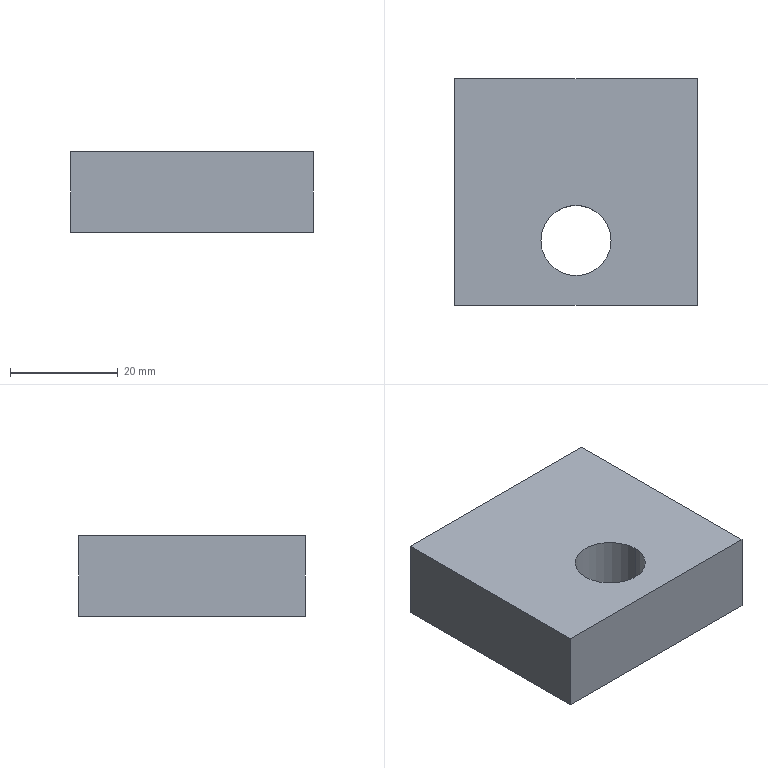Part | STEP file | adjusting block_default | 1 solid | 16 faces | box 45 x 42 x 15 mm | volume 24875 mm3 | cylinder 6 | plane 6 | cone 4 | commonest cylinder face diameters 6.8 x4 13 x2
STEP:
#1=CARTESIAN_POINT('',(0.,0.,0.));
#2=DIRECTION('',(0.,0.,1.));
#3=DIRECTION('',(1.,0.,0.));
#4=AXIS2_PLACEMENT_3D('',#1,#2,#3);
#5=CARTESIAN_POINT('',(29.,-30.,0.));
#6=VERTEX_POINT('',#5);
#7=CARTESIAN_POINT('',(29.,-30.,15.));
#8=VERTEX_POINT('',#7);
#9=CARTESIAN_POINT('',(29.,-30.,15.));
#10=DIRECTION('',(0.,0.,1.));
#11=VECTOR('',#10,1.);
#12=LINE('',#9,#11);
#13=CARTESIAN_POINT('',(22.5,-30.,15.));
#14=DIRECTION('',(0.,0.,1.));
#15=DIRECTION('',(1.,0.,0.));
#16=AXIS2_PLACEMENT_3D('',#13,#14,#15);
#17=CYLINDRICAL_SURFACE('',#16,6.5);
#18=CARTESIAN_POINT('',(6.283,0.));
#19=DIRECTION('',(0.,1.));
#20=VECTOR('',#19,1.);
#21=LINE('',#18,#20);
#22=(GEOMETRIC_REPRESENTATION_CONTEXT(2)PARAMETRIC_REPRESENTATION_CONTEXT()REPRESENTATION_CONTEXT('',''));
#23=DEFINITIONAL_REPRESENTATION('',(#21),#22);
#24=PCURVE('',#17,#23);
#25=CARTESIAN_POINT('',(22.5,-30.,15.));
#26=DIRECTION('',(0.,0.,1.));
#27=DIRECTION('',(1.,0.,0.));
#28=AXIS2_PLACEMENT_3D('',#25,#26,#27);
#29=CYLINDRICAL_SURFACE('',#28,6.5);
#30=CARTESIAN_POINT('',(0.,0.));
#31=DIRECTION('',(0.,1.));
#32=VECTOR('',#31,1.);
#33=LINE('',#30,#32);
#34=(GEOMETRIC_REPRESENTATION_CONTEXT(2)PARAMETRIC_REPRESENTATION_CONTEXT()REPRESENTATION_CONTEXT('',''));
#35=DEFINITIONAL_REPRESENTATION('',(#33),#34);
#36=PCURVE('',#29,#35);
#37=SURFACE_CURVE('',#12,(#24,#36),.PCURVE_S1.);
#38=EDGE_CURVE('',#6,#8,#37,.T.);
#39=ORIENTED_EDGE('',*,*,#38,.T.);
#40=CARTESIAN_POINT('',(16.,-30.,15.));
#41=VERTEX_POINT('',#40);
#42=CARTESIAN_POINT('',(22.5,-30.,15.));
#43=DIRECTION('',(0.,0.,1.));
#44=DIRECTION('',(1.,0.,0.));
#45=AXIS2_PLACEMENT_3D('',#42,#43,#44);
#46=CIRCLE('',#45,6.5);
#47=CARTESIAN_POINT('',(0.,0.));
#48=DIRECTION('',(1.,0.));
#49=VECTOR('',#48,1.);
#50=LINE('',#47,#49);
#51=(GEOMETRIC_REPRESENTATION_CONTEXT(2)PARAMETRIC_REPRESENTATION_CONTEXT()REPRESENTATION_CONTEXT('',''));
#52=DEFINITIONAL_REPRESENTATION('',(#50),#51);
#53=PCURVE('',#17,#52);
#54=CARTESIAN_POINT('',(0.,0.,15.));
#55=DIRECTION('',(0.,0.,1.));
#56=DIRECTION('',(1.,0.,0.));
#57=AXIS2_PLACEMENT_3D('',#54,#55,#56);
#58=PLANE('',#57);
#59=CARTESIAN_POINT('',(22.5,-30.));
#60=DIRECTION('',(1.,0.));
#61=AXIS2_PLACEMENT_2D('',#59,#60);
#62=CIRCLE('',#61,6.5);
#63=(GEOMETRIC_REPRESENTATION_CONTEXT(2)PARAMETRIC_REPRESENTATION_CONTEXT()REPRESENTATION_CONTEXT('',''));
#64=DEFINITIONAL_REPRESENTATION('',(#62),#63);
#65=PCURVE('',#58,#64);
#66=SURFACE_CURVE('',#46,(#53,#65),.PCURVE_S1.);
#67=EDGE_CURVE('',#41,#8,#66,.T.);
#68=ORIENTED_EDGE('',*,*,#67,.F.);
#69=CARTESIAN_POINT('',(16.,-30.,0.));
#70=VERTEX_POINT('',#69);
#71=CARTESIAN_POINT('',(16.,-30.,15.));
#72=DIRECTION('',(0.,0.,1.));
#73=VECTOR('',#72,1.);
#74=LINE('',#71,#73);
#75=CARTESIAN_POINT('',(3.142,0.));
#76=DIRECTION('',(0.,1.));
#77=VECTOR('',#76,1.);
#78=LINE('',#75,#77);
#79=(GEOMETRIC_REPRESENTATION_CONTEXT(2)PARAMETRIC_REPRESENTATION_CONTEXT()REPRESENTATION_CONTEXT('',''));
#80=DEFINITIONAL_REPRESENTATION('',(#78),#79);
#81=PCURVE('',#17,#80);
#82=CARTESIAN_POINT('',(3.142,0.));
#83=DIRECTION('',(0.,1.));
#84=VECTOR('',#83,1.);
#85=LINE('',#82,#84);
#86=(GEOMETRIC_REPRESENTATION_CONTEXT(2)PARAMETRIC_REPRESENTATION_CONTEXT()REPRESENTATION_CONTEXT('',''));
#87=DEFINITIONAL_REPRESENTATION('',(#85),#86);
#88=PCURVE('',#29,#87);
#89=SURFACE_CURVE('',#74,(#81,#88),.PCURVE_S1.);
#90=EDGE_CURVE('',#70,#41,#89,.T.);
#91=ORIENTED_EDGE('',*,*,#90,.F.);
#92=CARTESIAN_POINT('',(22.5,-30.,0.));
#93=DIRECTION('',(0.,0.,1.));
#94=DIRECTION('',(1.,0.,0.));
#95=AXIS2_PLACEMENT_3D('',#92,#93,#94);
#96=CIRCLE('',#95,6.5);
#97=CARTESIAN_POINT('',(0.,-15.));
#98=DIRECTION('',(1.,0.));
#99=VECTOR('',#98,1.);
#100=LINE('',#97,#99);
#101=(GEOMETRIC_REPRESENTATION_CONTEXT(2)PARAMETRIC_REPRESENTATION_CONTEXT()REPRESENTATION_CONTEXT('',''));
#102=DEFINITIONAL_REPRESENTATION('',(#100),#101);
#103=PCURVE('',#17,#102);
#104=CARTESIAN_POINT('',(0.,0.,0.));
#105=DIRECTION('',(0.,0.,1.));
#106=DIRECTION('',(1.,0.,0.));
#107=AXIS2_PLACEMENT_3D('',#104,#105,#106);
#108=PLANE('',#107);
#109=CARTESIAN_POINT('',(22.5,-30.));
#110=DIRECTION('',(1.,0.));
#111=AXIS2_PLACEMENT_2D('',#109,#110);
#112=CIRCLE('',#111,6.5);
#113=(GEOMETRIC_REPRESENTATION_CONTEXT(2)PARAMETRIC_REPRESENTATION_CONTEXT()REPRESENTATION_CONTEXT('',''));
#114=DEFINITIONAL_REPRESENTATION('',(#112),#113);
#115=PCURVE('',#108,#114);
#116=SURFACE_CURVE('',#96,(#103,#115),.PCURVE_S1.);
#117=EDGE_CURVE('',#70,#6,#116,.T.);
#118=ORIENTED_EDGE('',*,*,#117,.T.);
#119=EDGE_LOOP('',(#39,#68,#91,#118));
#120=FACE_BOUND('',#119,.F.);
#121=ADVANCED_FACE('',(#120),#17,.F.);
#122=CARTESIAN_POINT('',(7.5,-19.75,10.9));
#123=VERTEX_POINT('',#122);
#124=CARTESIAN_POINT('',(7.5,0.,10.9));
#125=VERTEX_POINT('',#124);
#126=CARTESIAN_POINT('',(7.5,0.,10.9));
#127=DIRECTION('',(0.,1.,0.));
#128=VECTOR('',#127,1.);
#129=LINE('',#126,#128);
#130=CARTESIAN_POINT('',(7.5,0.,7.5));
#131=DIRECTION('',(0.,1.,0.));
#132=DIRECTION('',(0.,0.,1.));
#133=AXIS2_PLACEMENT_3D('',#130,#131,#132);
#134=CYLINDRICAL_SURFACE('',#133,3.4);
#135=CARTESIAN_POINT('',(6.283,0.));
#136=DIRECTION('',(0.,1.));
#137=VECTOR('',#136,1.);
#138=LINE('',#135,#137);
#139=(GEOMETRIC_REPRESENTATION_CONTEXT(2)PARAMETRIC_REPRESENTATION_CONTEXT()REPRESENTATION_CONTEXT('',''));
#140=DEFINITIONAL_REPRESENTATION('',(#138),#139);
#141=PCURVE('',#134,#140);
#142=CARTESIAN_POINT('',(7.5,0.,7.5));
#143=DIRECTION('',(0.,1.,0.));
#144=DIRECTION('',(0.,0.,1.));
#145=AXIS2_PLACEMENT_3D('',#142,#143,#144);
#146=CYLINDRICAL_SURFACE('',#145,3.4);
#147=CARTESIAN_POINT('',(0.,0.));
#148=DIRECTION('',(0.,1.));
#149=VECTOR('',#148,1.);
#150=LINE('',#147,#149);
#151=(GEOMETRIC_REPRESENTATION_CONTEXT(2)PARAMETRIC_REPRESENTATION_CONTEXT()REPRESENTATION_CONTEXT('',''));
#152=DEFINITIONAL_REPRESENTATION('',(#150),#151);
#153=PCURVE('',#146,#152);
#154=SURFACE_CURVE('',#129,(#141,#153),.PCURVE_S1.);
#155=EDGE_CURVE('',#123,#125,#154,.T.);
#156=ORIENTED_EDGE('',*,*,#155,.T.);
#157=CARTESIAN_POINT('',(7.5,0.,4.1));
#158=VERTEX_POINT('',#157);
#159=CARTESIAN_POINT('',(7.5,0.,7.5));
#160=DIRECTION('',(0.,1.,0.));
#161=DIRECTION('',(0.,0.,1.));
#162=AXIS2_PLACEMENT_3D('',#159,#160,#161);
#163=CIRCLE('',#162,3.4);
#164=CARTESIAN_POINT('',(0.,0.));
#165=DIRECTION('',(1.,0.));
#166=VECTOR('',#165,1.);
#167=LINE('',#164,#166);
#168=(GEOMETRIC_REPRESENTATION_CONTEXT(2)PARAMETRIC_REPRESENTATION_CONTEXT()REPRESENTATION_CONTEXT('',''));
#169=DEFINITIONAL_REPRESENTATION('',(#167),#168);
#170=PCURVE('',#134,#169);
#171=CARTESIAN_POINT('',(0.,0.,15.));
#172=DIRECTION('',(0.,-1.,0.));
#173=DIRECTION('',(0.,0.,-1.));
#174=AXIS2_PLACEMENT_3D('',#171,#172,#173);
#175=PLANE('',#174);
#176=CARTESIAN_POINT('',(4.1,7.5));
#177=CARTESIAN_POINT('',(4.1,13.389));
#178=CARTESIAN_POINT('',(9.2,10.444));
#179=CARTESIAN_POINT('',(14.3,7.5));
#180=CARTESIAN_POINT('',(9.2,4.556));
#181=CARTESIAN_POINT('',(4.1,1.611));
#182=CARTESIAN_POINT('',(4.1,7.5));
#183=(BOUNDED_CURVE()B_SPLINE_CURVE(2,(#176,#177,#178,#179,#180,#181,#182),.UNSPECIFIED.,.T.,.F.)B_SPLINE_CURVE_WITH_KNOTS((1,2,2,2,2,1),(-2.094,0.,2.094,4.189,6.283,8.378),.UNSPECIFIED.)CURVE()GEOMETRIC_REPRESENTATION_ITEM()RATIONAL_B_SPLINE_CURVE((1.,0.5,1.,0.5,1.,0.5,1.))REPRESENTATION_ITEM(''));
#184=(GEOMETRIC_REPRESENTATION_CONTEXT(2)PARAMETRIC_REPRESENTATION_CONTEXT()REPRESENTATION_CONTEXT('',''));
#185=DEFINITIONAL_REPRESENTATION('',(#183),#184);
#186=PCURVE('',#175,#185);
#187=SURFACE_CURVE('',#163,(#170,#186),.PCURVE_S1.);
#188=EDGE_CURVE('',#158,#125,#187,.T.);
#189=ORIENTED_EDGE('',*,*,#188,.F.);
#190=CARTESIAN_POINT('',(7.5,-19.75,4.1));
#191=VERTEX_POINT('',#190);
#192=CARTESIAN_POINT('',(7.5,0.,4.1));
#193=DIRECTION('',(0.,1.,0.));
#194=VECTOR('',#193,1.);
#195=LINE('',#192,#194);
#196=CARTESIAN_POINT('',(3.142,0.));
#197=DIRECTION('',(0.,1.));
#198=VECTOR('',#197,1.);
#199=LINE('',#196,#198);
#200=(GEOMETRIC_REPRESENTATION_CONTEXT(2)PARAMETRIC_REPRESENTATION_CONTEXT()REPRESENTATION_CONTEXT('',''));
#201=DEFINITIONAL_REPRESENTATION('',(#199),#200);
#202=PCURVE('',#134,#201);
#203=CARTESIAN_POINT('',(3.142,0.));
#204=DIRECTION('',(0.,1.));
#205=VECTOR('',#204,1.);
#206=LINE('',#203,#205);
#207=(GEOMETRIC_REPRESENTATION_CONTEXT(2)PARAMETRIC_REPRESENTATION_CONTEXT()REPRESENTATION_CONTEXT('',''));
#208=DEFINITIONAL_REPRESENTATION('',(#206),#207);
#209=PCURVE('',#146,#208);
#210=SURFACE_CURVE('',#195,(#202,#209),.PCURVE_S1.);
#211=EDGE_CURVE('',#191,#158,#210,.T.);
#212=ORIENTED_EDGE('',*,*,#211,.F.);
#213=CARTESIAN_POINT('',(7.5,-19.75,7.5));
#214=DIRECTION('',(0.,1.,0.));
#215=DIRECTION('',(0.,0.,1.));
#216=AXIS2_PLACEMENT_3D('',#213,#214,#215);
#217=CIRCLE('',#216,3.4);
#218=CARTESIAN_POINT('',(0.,-19.75));
#219=DIRECTION('',(1.,0.));
#220=VECTOR('',#219,1.);
#221=LINE('',#218,#220);
#222=(GEOMETRIC_REPRESENTATION_CONTEXT(2)PARAMETRIC_REPRESENTATION_CONTEXT()REPRESENTATION_CONTEXT('',''));
#223=DEFINITIONAL_REPRESENTATION('',(#221),#222);
#224=PCURVE('',#134,#223);
#225=CARTESIAN_POINT('',(7.5,-19.75,7.5));
#226=DIRECTION('',(0.,1.,0.));
#227=DIRECTION('',(0.,0.,1.));
#228=AXIS2_PLACEMENT_3D('',#225,#226,#227);
#229=CONICAL_SURFACE('',#228,3.4,1.03);
#230=CARTESIAN_POINT('',(0.,0.));
#231=DIRECTION('',(1.,0.));
#232=VECTOR('',#231,1.);
#233=LINE('',#230,#232);
#234=(GEOMETRIC_REPRESENTATION_CONTEXT(2)PARAMETRIC_REPRESENTATION_CONTEXT()REPRESENTATION_CONTEXT('',''));
#235=DEFINITIONAL_REPRESENTATION('',(#233),#234);
#236=PCURVE('',#229,#235);
#237=SURFACE_CURVE('',#217,(#224,#236),.PCURVE_S1.);
#238=EDGE_CURVE('',#191,#123,#237,.T.);
#239=ORIENTED_EDGE('',*,*,#238,.T.);
#240=EDGE_LOOP('',(#156,#189,#212,#239));
#241=FACE_BOUND('',#240,.F.);
#242=ADVANCED_FACE('',(#241),#134,.F.);
#243=ORIENTED_EDGE('',*,*,#238,.F.);
#244=CARTESIAN_POINT('',(7.5,-21.793,7.5));
#245=VERTEX_POINT('',#244);
#246=CARTESIAN_POINT('',(7.5,-19.75,4.1));
#247=DIRECTION('',(0.,0.515,-0.8572));
#248=VECTOR('',#247,1.);
#249=LINE('',#246,#248);
#250=CARTESIAN_POINT('',(3.142,0.));
#251=DIRECTION('',(0.,1.));
#252=VECTOR('',#251,1.);
#253=LINE('',#250,#252);
#254=(GEOMETRIC_REPRESENTATION_CONTEXT(2)PARAMETRIC_REPRESENTATION_CONTEXT()REPRESENTATION_CONTEXT('',''));
#255=DEFINITIONAL_REPRESENTATION('',(#253),#254);
#256=PCURVE('',#229,#255);
#257=CARTESIAN_POINT('',(7.5,-19.75,7.5));
#258=DIRECTION('',(0.,1.,0.));
#259=DIRECTION('',(0.,0.,1.));
#260=AXIS2_PLACEMENT_3D('',#257,#258,#259);
#261=CONICAL_SURFACE('',#260,3.4,1.03);
#262=CARTESIAN_POINT('',(3.142,0.));
#263=DIRECTION('',(0.,1.));
#264=VECTOR('',#263,1.);
#265=LINE('',#262,#264);
#266=(GEOMETRIC_REPRESENTATION_CONTEXT(2)PARAMETRIC_REPRESENTATION_CONTEXT()REPRESENTATION_CONTEXT('',''));
#267=DEFINITIONAL_REPRESENTATION('',(#265),#266);
#268=PCURVE('',#261,#267);
#269=SURFACE_CURVE('',#249,(#256,#268),.PCURVE_S1.);
#270=EDGE_CURVE('',#245,#191,#269,.T.);
#271=ORIENTED_EDGE('',*,*,#270,.F.);
#272=CARTESIAN_POINT('',(7.5,-19.75,10.9));
#273=DIRECTION('',(0.,0.515,0.8572));
#274=VECTOR('',#273,1.);
#275=LINE('',#272,#274);
#276=CARTESIAN_POINT('',(6.283,0.));
#277=DIRECTION('',(0.,1.));
#278=VECTOR('',#277,1.);
#279=LINE('',#276,#278);
#280=(GEOMETRIC_REPRESENTATION_CONTEXT(2)PARAMETRIC_REPRESENTATION_CONTEXT()REPRESENTATION_CONTEXT('',''));
#281=DEFINITIONAL_REPRESENTATION('',(#279),#280);
#282=PCURVE('',#229,#281);
#283=CARTESIAN_POINT('',(0.,0.));
#284=DIRECTION('',(0.,1.));
#285=VECTOR('',#284,1.);
#286=LINE('',#283,#285);
#287=(GEOMETRIC_REPRESENTATION_CONTEXT(2)PARAMETRIC_REPRESENTATION_CONTEXT()REPRESENTATION_CONTEXT('',''));
#288=DEFINITIONAL_REPRESENTATION('',(#286),#287);
#289=PCURVE('',#261,#288);
#290=SURFACE_CURVE('',#275,(#282,#289),.PCURVE_S1.);
#291=EDGE_CURVE('',#245,#123,#290,.T.);
#292=ORIENTED_EDGE('',*,*,#291,.T.);
#293=EDGE_LOOP('',(#243,#271,#292));
#294=FACE_BOUND('',#293,.F.);
#295=ADVANCED_FACE('',(#294),#229,.F.);
#296=CARTESIAN_POINT('',(37.5,-19.75,10.9));
#297=VERTEX_POINT('',#296);
#298=CARTESIAN_POINT('',(37.5,0.,10.9));
#299=VERTEX_POINT('',#298);
#300=CARTESIAN_POINT('',(37.5,0.,10.9));
#301=DIRECTION('',(0.,1.,0.));
#302=VECTOR('',#301,1.);
#303=LINE('',#300,#302);
#304=CARTESIAN_POINT('',(37.5,0.,7.5));
#305=DIRECTION('',(0.,1.,0.));
#306=DIRECTION('',(0.,0.,1.));
#307=AXIS2_PLACEMENT_3D('',#304,#305,#306);
#308=CYLINDRICAL_SURFACE('',#307,3.4);
#309=CARTESIAN_POINT('',(6.283,0.));
#310=DIRECTION('',(0.,1.));
#311=VECTOR('',#310,1.);
#312=LINE('',#309,#311);
#313=(GEOMETRIC_REPRESENTATION_CONTEXT(2)PARAMETRIC_REPRESENTATION_CONTEXT()REPRESENTATION_CONTEXT('',''));
#314=DEFINITIONAL_REPRESENTATION('',(#312),#313);
#315=PCURVE('',#308,#314);
#316=CARTESIAN_POINT('',(37.5,0.,7.5));
#317=DIRECTION('',(0.,1.,0.));
#318=DIRECTION('',(0.,0.,1.));
#319=AXIS2_PLACEMENT_3D('',#316,#317,#318);
#320=CYLINDRICAL_SURFACE('',#319,3.4);
#321=CARTESIAN_POINT('',(0.,0.));
#322=DIRECTION('',(0.,1.));
#323=VECTOR('',#322,1.);
#324=LINE('',#321,#323);
#325=(GEOMETRIC_REPRESENTATION_CONTEXT(2)PARAMETRIC_REPRESENTATION_CONTEXT()REPRESENTATION_CONTEXT('',''));
#326=DEFINITIONAL_REPRESENTATION('',(#324),#325);
#327=PCURVE('',#320,#326);
#328=SURFACE_CURVE('',#303,(#315,#327),.PCURVE_S1.);
#329=EDGE_CURVE('',#297,#299,#328,.T.);
#330=ORIENTED_EDGE('',*,*,#329,.T.);
#331=CARTESIAN_POINT('',(37.5,0.,4.1));
#332=VERTEX_POINT('',#331);
#333=CARTESIAN_POINT('',(37.5,0.,7.5));
#334=DIRECTION('',(0.,1.,0.));
#335=DIRECTION('',(0.,0.,1.));
#336=AXIS2_PLACEMENT_3D('',#333,#334,#335);
#337=CIRCLE('',#336,3.4);
#338=CARTESIAN_POINT('',(0.,0.));
#339=DIRECTION('',(1.,0.));
#340=VECTOR('',#339,1.);
#341=LINE('',#338,#340);
#342=(GEOMETRIC_REPRESENTATION_CONTEXT(2)PARAMETRIC_REPRESENTATION_CONTEXT()REPRESENTATION_CONTEXT('',''));
#343=DEFINITIONAL_REPRESENTATION('',(#341),#342);
#344=PCURVE('',#308,#343);
#345=CARTESIAN_POINT('',(4.1,37.5));
#346=CARTESIAN_POINT('',(4.1,43.389));
#347=CARTESIAN_POINT('',(9.2,40.444));
#348=CARTESIAN_POINT('',(14.3,37.5));
#349=CARTESIAN_POINT('',(9.2,34.556));
#350=CARTESIAN_POINT('',(4.1,31.611));
#351=CARTESIAN_POINT('',(4.1,37.5));
#352=(BOUNDED_CURVE()B_SPLINE_CURVE(2,(#345,#346,#347,#348,#349,#350,#351),.UNSPECIFIED.,.T.,.F.)B_SPLINE_CURVE_WITH_KNOTS((1,2,2,2,2,1),(-2.094,0.,2.094,4.189,6.283,8.378),.UNSPECIFIED.)CURVE()GEOMETRIC_REPRESENTATION_ITEM()RATIONAL_B_SPLINE_CURVE((1.,0.5,1.,0.5,1.,0.5,1.))REPRESENTATION_ITEM(''));
#353=(GEOMETRIC_REPRESENTATION_CONTEXT(2)PARAMETRIC_REPRESENTATION_CONTEXT()REPRESENTATION_CONTEXT('',''));
#354=DEFINITIONAL_REPRESENTATION('',(#352),#353);
#355=PCURVE('',#175,#354);
#356=SURFACE_CURVE('',#337,(#344,#355),.PCURVE_S1.);
#357=EDGE_CURVE('',#332,#299,#356,.T.);
#358=ORIENTED_EDGE('',*,*,#357,.F.);
#359=CARTESIAN_POINT('',(37.5,-19.75,4.1));
#360=VERTEX_POINT('',#359);
#361=CARTESIAN_POINT('',(37.5,0.,4.1));
#362=DIRECTION('',(0.,1.,0.));
#363=VECTOR('',#362,1.);
#364=LINE('',#361,#363);
#365=CARTESIAN_POINT('',(3.142,0.));
#366=DIRECTION('',(0.,1.));
#367=VECTOR('',#366,1.);
#368=LINE('',#365,#367);
#369=(GEOMETRIC_REPRESENTATION_CONTEXT(2)PARAMETRIC_REPRESENTATION_CONTEXT()REPRESENTATION_CONTEXT('',''));
#370=DEFINITIONAL_REPRESENTATION('',(#368),#369);
#371=PCURVE('',#308,#370);
#372=CARTESIAN_POINT('',(3.142,0.));
#373=DIRECTION('',(0.,1.));
#374=VECTOR('',#373,1.);
#375=LINE('',#372,#374);
#376=(GEOMETRIC_REPRESENTATION_CONTEXT(2)PARAMETRIC_REPRESENTATION_CONTEXT()REPRESENTATION_CONTEXT('',''));
#377=DEFINITIONAL_REPRESENTATION('',(#375),#376);
#378=PCURVE('',#320,#377);
#379=SURFACE_CURVE('',#364,(#371,#378),.PCURVE_S1.);
#380=EDGE_CURVE('',#360,#332,#379,.T.);
#381=ORIENTED_EDGE('',*,*,#380,.F.);
#382=CARTESIAN_POINT('',(37.5,-19.75,7.5));
#383=DIRECTION('',(0.,1.,0.));
#384=DIRECTION('',(0.,0.,1.));
#385=AXIS2_PLACEMENT_3D('',#382,#383,#384);
#386=CIRCLE('',#385,3.4);
#387=CARTESIAN_POINT('',(0.,-19.75));
#388=DIRECTION('',(1.,0.));
#389=VECTOR('',#388,1.);
#390=LINE('',#387,#389);
#391=(GEOMETRIC_REPRESENTATION_CONTEXT(2)PARAMETRIC_REPRESENTATION_CONTEXT()REPRESENTATION_CONTEXT('',''));
#392=DEFINITIONAL_REPRESENTATION('',(#390),#391);
#393=PCURVE('',#308,#392);
#394=CARTESIAN_POINT('',(37.5,-19.75,7.5));
#395=DIRECTION('',(0.,1.,0.));
#396=DIRECTION('',(0.,0.,1.));
#397=AXIS2_PLACEMENT_3D('',#394,#395,#396);
#398=CONICAL_SURFACE('',#397,3.4,1.03);
#399=CARTESIAN_POINT('',(0.,0.));
#400=DIRECTION('',(1.,0.));
#401=VECTOR('',#400,1.);
#402=LINE('',#399,#401);
#403=(GEOMETRIC_REPRESENTATION_CONTEXT(2)PARAMETRIC_REPRESENTATION_CONTEXT()REPRESENTATION_CONTEXT('',''));
#404=DEFINITIONAL_REPRESENTATION('',(#402),#403);
#405=PCURVE('',#398,#404);
#406=SURFACE_CURVE('',#386,(#393,#405),.PCURVE_S1.);
#407=EDGE_CURVE('',#360,#297,#406,.T.);
#408=ORIENTED_EDGE('',*,*,#407,.T.);
#409=EDGE_LOOP('',(#330,#358,#381,#408));
#410=FACE_BOUND('',#409,.F.);
#411=ADVANCED_FACE('',(#410),#308,.F.);
#412=ORIENTED_EDGE('',*,*,#407,.F.);
#413=CARTESIAN_POINT('',(37.5,-21.793,7.5));
#414=VERTEX_POINT('',#413);
#415=CARTESIAN_POINT('',(37.5,-19.75,4.1));
#416=DIRECTION('',(0.,0.515,-0.8572));
#417=VECTOR('',#416,1.);
#418=LINE('',#415,#417);
#419=CARTESIAN_POINT('',(3.142,0.));
#420=DIRECTION('',(0.,1.));
#421=VECTOR('',#420,1.);
#422=LINE('',#419,#421);
#423=(GEOMETRIC_REPRESENTATION_CONTEXT(2)PARAMETRIC_REPRESENTATION_CONTEXT()REPRESENTATION_CONTEXT('',''));
#424=DEFINITIONAL_REPRESENTATION('',(#422),#423);
#425=PCURVE('',#398,#424);
#426=CARTESIAN_POINT('',(37.5,-19.75,7.5));
#427=DIRECTION('',(0.,1.,0.));
#428=DIRECTION('',(0.,0.,1.));
#429=AXIS2_PLACEMENT_3D('',#426,#427,#428);
#430=CONICAL_SURFACE('',#429,3.4,1.03);
#431=CARTESIAN_POINT('',(3.142,0.));
#432=DIRECTION('',(0.,1.));
#433=VECTOR('',#432,1.);
#434=LINE('',#431,#433);
#435=(GEOMETRIC_REPRESENTATION_CONTEXT(2)PARAMETRIC_REPRESENTATION_CONTEXT()REPRESENTATION_CONTEXT('',''));
#436=DEFINITIONAL_REPRESENTATION('',(#434),#435);
#437=PCURVE('',#430,#436);
#438=SURFACE_CURVE('',#418,(#425,#437),.PCURVE_S1.);
#439=EDGE_CURVE('',#414,#360,#438,.T.);
#440=ORIENTED_EDGE('',*,*,#439,.F.);
#441=CARTESIAN_POINT('',(37.5,-19.75,10.9));
#442=DIRECTION('',(0.,0.515,0.8572));
#443=VECTOR('',#442,1.);
#444=LINE('',#441,#443);
#445=CARTESIAN_POINT('',(6.283,0.));
#446=DIRECTION('',(0.,1.));
#447=VECTOR('',#446,1.);
#448=LINE('',#445,#447);
#449=(GEOMETRIC_REPRESENTATION_CONTEXT(2)PARAMETRIC_REPRESENTATION_CONTEXT()REPRESENTATION_CONTEXT('',''));
#450=DEFINITIONAL_REPRESENTATION('',(#448),#449);
#451=PCURVE('',#398,#450);
#452=CARTESIAN_POINT('',(0.,0.));
#453=DIRECTION('',(0.,1.));
#454=VECTOR('',#453,1.);
#455=LINE('',#452,#454);
#456=(GEOMETRIC_REPRESENTATION_CONTEXT(2)PARAMETRIC_REPRESENTATION_CONTEXT()REPRESENTATION_CONTEXT('',''));
#457=DEFINITIONAL_REPRESENTATION('',(#455),#456);
#458=PCURVE('',#430,#457);
#459=SURFACE_CURVE('',#444,(#451,#458),.PCURVE_S1.);
#460=EDGE_CURVE('',#414,#297,#459,.T.);
#461=ORIENTED_EDGE('',*,*,#460,.T.);
#462=EDGE_LOOP('',(#412,#440,#461));
#463=FACE_BOUND('',#462,.F.);
#464=ADVANCED_FACE('',(#463),#398,.F.);
#465=CARTESIAN_POINT('',(0.,0.,0.));
#466=VERTEX_POINT('',#465);
#467=CARTESIAN_POINT('',(0.,-42.,0.));
#468=VERTEX_POINT('',#467);
#469=CARTESIAN_POINT('',(0.,0.,0.));
#470=DIRECTION('',(0.,-1.,0.));
#471=VECTOR('',#470,1.);
#472=LINE('',#469,#471);
#473=CARTESIAN_POINT('',(0.,0.,15.));
#474=DIRECTION('',(1.,0.,0.));
#475=DIRECTION('',(0.,1.,0.));
#476=AXIS2_PLACEMENT_3D('',#473,#474,#475);
#477=PLANE('',#476);
#478=CARTESIAN_POINT('',(0.,-15.));
#479=DIRECTION('',(-1.,0.));
#480=VECTOR('',#479,1.);
#481=LINE('',#478,#480);
#482=(GEOMETRIC_REPRESENTATION_CONTEXT(2)PARAMETRIC_REPRESENTATION_CONTEXT()REPRESENTATION_CONTEXT('',''));
#483=DEFINITIONAL_REPRESENTATION('',(#481),#482);
#484=PCURVE('',#477,#483);
#485=CARTESIAN_POINT('',(0.,0.));
#486=DIRECTION('',(0.,-1.));
#487=VECTOR('',#486,1.);
#488=LINE('',#485,#487);
#489=(GEOMETRIC_REPRESENTATION_CONTEXT(2)PARAMETRIC_REPRESENTATION_CONTEXT()REPRESENTATION_CONTEXT('',''));
#490=DEFINITIONAL_REPRESENTATION('',(#488),#489);
#491=PCURVE('',#108,#490);
#492=SURFACE_CURVE('',#472,(#484,#491),.PCURVE_S1.);
#493=EDGE_CURVE('',#466,#468,#492,.T.);
#494=ORIENTED_EDGE('',*,*,#493,.T.);
#495=CARTESIAN_POINT('',(0.,-42.,15.));
#496=VERTEX_POINT('',#495);
#497=CARTESIAN_POINT('',(0.,-42.,15.));
#498=DIRECTION('',(0.,0.,-1.));
#499=VECTOR('',#498,1.);
#500=LINE('',#497,#499);
#501=CARTESIAN_POINT('',(-42.,0.));
#502=DIRECTION('',(0.,-1.));
#503=VECTOR('',#502,1.);
#504=LINE('',#501,#503);
#505=(GEOMETRIC_REPRESENTATION_CONTEXT(2)PARAMETRIC_REPRESENTATION_CONTEXT()REPRESENTATION_CONTEXT('',''));
#506=DEFINITIONAL_REPRESENTATION('',(#504),#505);
#507=PCURVE('',#477,#506);
#508=CARTESIAN_POINT('',(0.,-42.,15.));
#509=DIRECTION('',(0.,1.,0.));
#510=DIRECTION('',(0.,0.,1.));
#511=AXIS2_PLACEMENT_3D('',#508,#509,#510);
#512=PLANE('',#511);
#513=CARTESIAN_POINT('',(0.,0.));
#514=DIRECTION('',(-1.,0.));
#515=VECTOR('',#514,1.);
#516=LINE('',#513,#515);
#517=(GEOMETRIC_REPRESENTATION_CONTEXT(2)PARAMETRIC_REPRESENTATION_CONTEXT()REPRESENTATION_CONTEXT('',''));
#518=DEFINITIONAL_REPRESENTATION('',(#516),#517);
#519=PCURVE('',#512,#518);
#520=SURFACE_CURVE('',#500,(#507,#519),.PCURVE_S1.);
#521=EDGE_CURVE('',#496,#468,#520,.T.);
#522=ORIENTED_EDGE('',*,*,#521,.F.);
#523=CARTESIAN_POINT('',(0.,0.,15.));
#524=VERTEX_POINT('',#523);
#525=CARTESIAN_POINT('',(0.,0.,15.));
#526=DIRECTION('',(0.,-1.,0.));
#527=VECTOR('',#526,1.);
#528=LINE('',#525,#527);
#529=CARTESIAN_POINT('',(0.,0.));
#530=DIRECTION('',(-1.,0.));
#531=VECTOR('',#530,1.);
#532=LINE('',#529,#531);
#533=(GEOMETRIC_REPRESENTATION_CONTEXT(2)PARAMETRIC_REPRESENTATION_CONTEXT()REPRESENTATION_CONTEXT('',''));
#534=DEFINITIONAL_REPRESENTATION('',(#532),#533);
#535=PCURVE('',#477,#534);
#536=CARTESIAN_POINT('',(0.,0.));
#537=DIRECTION('',(0.,-1.));
#538=VECTOR('',#537,1.);
#539=LINE('',#536,#538);
#540=(GEOMETRIC_REPRESENTATION_CONTEXT(2)PARAMETRIC_REPRESENTATION_CONTEXT()REPRESENTATION_CONTEXT('',''));
#541=DEFINITIONAL_REPRESENTATION('',(#539),#540);
#542=PCURVE('',#58,#541);
#543=SURFACE_CURVE('',#528,(#535,#542),.PCURVE_S1.);
#544=EDGE_CURVE('',#524,#496,#543,.T.);
#545=ORIENTED_EDGE('',*,*,#544,.F.);
#546=CARTESIAN_POINT('',(0.,0.,15.));
#547=DIRECTION('',(0.,0.,-1.));
#548=VECTOR('',#547,1.);
#549=LINE('',#546,#548);
#550=CARTESIAN_POINT('',(0.,0.));
#551=DIRECTION('',(0.,-1.));
#552=VECTOR('',#551,1.);
#553=LINE('',#550,#552);
#554=(GEOMETRIC_REPRESENTATION_CONTEXT(2)PARAMETRIC_REPRESENTATION_CONTEXT()REPRESENTATION_CONTEXT('',''));
#555=DEFINITIONAL_REPRESENTATION('',(#553),#554);
#556=PCURVE('',#477,#555);
#557=CARTESIAN_POINT('',(0.,0.));
#558=DIRECTION('',(1.,0.));
#559=VECTOR('',#558,1.);
#560=LINE('',#557,#559);
#561=(GEOMETRIC_REPRESENTATION_CONTEXT(2)PARAMETRIC_REPRESENTATION_CONTEXT()REPRESENTATION_CONTEXT('',''));
#562=DEFINITIONAL_REPRESENTATION('',(#560),#561);
#563=PCURVE('',#175,#562);
#564=SURFACE_CURVE('',#549,(#556,#563),.PCURVE_S1.);
#565=EDGE_CURVE('',#524,#466,#564,.T.);
#566=ORIENTED_EDGE('',*,*,#565,.T.);
#567=EDGE_LOOP('',(#494,#522,#545,#566));
#568=FACE_BOUND('',#567,.T.);
#569=ADVANCED_FACE('',(#568),#477,.F.);
#570=CARTESIAN_POINT('',(45.,-42.,0.));
#571=VERTEX_POINT('',#570);
#572=CARTESIAN_POINT('',(0.,-42.,0.));
#573=DIRECTION('',(1.,0.,0.));
#574=VECTOR('',#573,1.);
#575=LINE('',#572,#574);
#576=CARTESIAN_POINT('',(-15.,0.));
#577=DIRECTION('',(0.,1.));
#578=VECTOR('',#577,1.);
#579=LINE('',#576,#578);
#580=(GEOMETRIC_REPRESENTATION_CONTEXT(2)PARAMETRIC_REPRESENTATION_CONTEXT()REPRESENTATION_CONTEXT('',''));
#581=DEFINITIONAL_REPRESENTATION('',(#579),#580);
#582=PCURVE('',#512,#581);
#583=CARTESIAN_POINT('',(0.,-42.));
#584=DIRECTION('',(1.,0.));
#585=VECTOR('',#584,1.);
#586=LINE('',#583,#585);
#587=(GEOMETRIC_REPRESENTATION_CONTEXT(2)PARAMETRIC_REPRESENTATION_CONTEXT()REPRESENTATION_CONTEXT('',''));
#588=DEFINITIONAL_REPRESENTATION('',(#586),#587);
#589=PCURVE('',#108,#588);
#590=SURFACE_CURVE('',#575,(#582,#589),.PCURVE_S1.);
#591=EDGE_CURVE('',#468,#571,#590,.T.);
#592=ORIENTED_EDGE('',*,*,#591,.T.);
#593=CARTESIAN_POINT('',(45.,-42.,15.));
#594=VERTEX_POINT('',#593);
#595=CARTESIAN_POINT('',(45.,-42.,15.));
#596=DIRECTION('',(0.,0.,-1.));
#597=VECTOR('',#596,1.);
#598=LINE('',#595,#597);
#599=CARTESIAN_POINT('',(0.,45.));
#600=DIRECTION('',(-1.,0.));
#601=VECTOR('',#600,1.);
#602=LINE('',#599,#601);
#603=(GEOMETRIC_REPRESENTATION_CONTEXT(2)PARAMETRIC_REPRESENTATION_CONTEXT()REPRESENTATION_CONTEXT('',''));
#604=DEFINITIONAL_REPRESENTATION('',(#602),#603);
#605=PCURVE('',#512,#604);
#606=CARTESIAN_POINT('',(45.,0.,15.));
#607=DIRECTION('',(-1.,0.,0.));
#608=DIRECTION('',(0.,0.,1.));
#609=AXIS2_PLACEMENT_3D('',#606,#607,#608);
#610=PLANE('',#609);
#611=CARTESIAN_POINT('',(0.,-42.));
#612=DIRECTION('',(-1.,0.));
#613=VECTOR('',#612,1.);
#614=LINE('',#611,#613);
#615=(GEOMETRIC_REPRESENTATION_CONTEXT(2)PARAMETRIC_REPRESENTATION_CONTEXT()REPRESENTATION_CONTEXT('',''));
#616=DEFINITIONAL_REPRESENTATION('',(#614),#615);
#617=PCURVE('',#610,#616);
#618=SURFACE_CURVE('',#598,(#605,#617),.PCURVE_S1.);
#619=EDGE_CURVE('',#594,#571,#618,.T.);
#620=ORIENTED_EDGE('',*,*,#619,.F.);
#621=CARTESIAN_POINT('',(0.,-42.,15.));
#622=DIRECTION('',(1.,0.,0.));
#623=VECTOR('',#622,1.);
#624=LINE('',#621,#623);
#625=CARTESIAN_POINT('',(0.,0.));
#626=DIRECTION('',(0.,1.));
#627=VECTOR('',#626,1.);
#628=LINE('',#625,#627);
#629=(GEOMETRIC_REPRESENTATION_CONTEXT(2)PARAMETRIC_REPRESENTATION_CONTEXT()REPRESENTATION_CONTEXT('',''));
#630=DEFINITIONAL_REPRESENTATION('',(#628),#629);
#631=PCURVE('',#512,#630);
#632=CARTESIAN_POINT('',(0.,-42.));
#633=DIRECTION('',(1.,0.));
#634=VECTOR('',#633,1.);
#635=LINE('',#632,#634);
#636=(GEOMETRIC_REPRESENTATION_CONTEXT(2)PARAMETRIC_REPRESENTATION_CONTEXT()REPRESENTATION_CONTEXT('',''));
#637=DEFINITIONAL_REPRESENTATION('',(#635),#636);
#638=PCURVE('',#58,#637);
#639=SURFACE_CURVE('',#624,(#631,#638),.PCURVE_S1.);
#640=EDGE_CURVE('',#496,#594,#639,.T.);
#641=ORIENTED_EDGE('',*,*,#640,.F.);
#642=ORIENTED_EDGE('',*,*,#521,.T.);
#643=EDGE_LOOP('',(#592,#620,#641,#642));
#644=FACE_BOUND('',#643,.T.);
#645=ADVANCED_FACE('',(#644),#512,.F.);
#646=CARTESIAN_POINT('',(45.,0.,0.));
#647=VERTEX_POINT('',#646);
#648=CARTESIAN_POINT('',(45.,0.,0.));
#649=DIRECTION('',(0.,1.,0.));
#650=VECTOR('',#649,1.);
#651=LINE('',#648,#650);
#652=CARTESIAN_POINT('',(-15.,0.));
#653=DIRECTION('',(0.,1.));
#654=VECTOR('',#653,1.);
#655=LINE('',#652,#654);
#656=(GEOMETRIC_REPRESENTATION_CONTEXT(2)PARAMETRIC_REPRESENTATION_CONTEXT()REPRESENTATION_CONTEXT('',''));
#657=DEFINITIONAL_REPRESENTATION('',(#655),#656);
#658=PCURVE('',#610,#657);
#659=CARTESIAN_POINT('',(45.,0.));
#660=DIRECTION('',(0.,1.));
#661=VECTOR('',#660,1.);
#662=LINE('',#659,#661);
#663=(GEOMETRIC_REPRESENTATION_CONTEXT(2)PARAMETRIC_REPRESENTATION_CONTEXT()REPRESENTATION_CONTEXT('',''));
#664=DEFINITIONAL_REPRESENTATION('',(#662),#663);
#665=PCURVE('',#108,#664);
#666=SURFACE_CURVE('',#651,(#658,#665),.PCURVE_S1.);
#667=EDGE_CURVE('',#571,#647,#666,.T.);
#668=ORIENTED_EDGE('',*,*,#667,.T.);
#669=CARTESIAN_POINT('',(45.,0.,15.));
#670=VERTEX_POINT('',#669);
#671=CARTESIAN_POINT('',(45.,0.,15.));
#672=DIRECTION('',(0.,0.,-1.));
#673=VECTOR('',#672,1.);
#674=LINE('',#671,#673);
#675=CARTESIAN_POINT('',(0.,0.));
#676=DIRECTION('',(-1.,0.));
#677=VECTOR('',#676,1.);
#678=LINE('',#675,#677);
#679=(GEOMETRIC_REPRESENTATION_CONTEXT(2)PARAMETRIC_REPRESENTATION_CONTEXT()REPRESENTATION_CONTEXT('',''));
#680=DEFINITIONAL_REPRESENTATION('',(#678),#679);
#681=PCURVE('',#610,#680);
#682=CARTESIAN_POINT('',(0.,45.));
#683=DIRECTION('',(1.,0.));
#684=VECTOR('',#683,1.);
#685=LINE('',#682,#684);
#686=(GEOMETRIC_REPRESENTATION_CONTEXT(2)PARAMETRIC_REPRESENTATION_CONTEXT()REPRESENTATION_CONTEXT('',''));
#687=DEFINITIONAL_REPRESENTATION('',(#685),#686);
#688=PCURVE('',#175,#687);
#689=SURFACE_CURVE('',#674,(#681,#688),.PCURVE_S1.);
#690=EDGE_CURVE('',#670,#647,#689,.T.);
#691=ORIENTED_EDGE('',*,*,#690,.F.);
#692=CARTESIAN_POINT('',(45.,0.,15.));
#693=DIRECTION('',(0.,1.,0.));
#694=VECTOR('',#693,1.);
#695=LINE('',#692,#694);
#696=CARTESIAN_POINT('',(0.,0.));
#697=DIRECTION('',(0.,1.));
#698=VECTOR('',#697,1.);
#699=LINE('',#696,#698);
#700=(GEOMETRIC_REPRESENTATION_CONTEXT(2)PARAMETRIC_REPRESENTATION_CONTEXT()REPRESENTATION_CONTEXT('',''));
#701=DEFINITIONAL_REPRESENTATION('',(#699),#700);
#702=PCURVE('',#610,#701);
#703=CARTESIAN_POINT('',(45.,0.));
#704=DIRECTION('',(0.,1.));
#705=VECTOR('',#704,1.);
#706=LINE('',#703,#705);
#707=(GEOMETRIC_REPRESENTATION_CONTEXT(2)PARAMETRIC_REPRESENTATION_CONTEXT()REPRESENTATION_CONTEXT('',''));
#708=DEFINITIONAL_REPRESENTATION('',(#706),#707);
#709=PCURVE('',#58,#708);
#710=SURFACE_CURVE('',#695,(#702,#709),.PCURVE_S1.);
#711=EDGE_CURVE('',#594,#670,#710,.T.);
#712=ORIENTED_EDGE('',*,*,#711,.F.);
#713=ORIENTED_EDGE('',*,*,#619,.T.);
#714=EDGE_LOOP('',(#668,#691,#712,#713));
#715=FACE_BOUND('',#714,.T.);
#716=ADVANCED_FACE('',(#715),#610,.F.);
#717=CARTESIAN_POINT('',(7.5,0.,7.5));
#718=DIRECTION('',(0.,1.,0.));
#719=DIRECTION('',(0.,0.,1.));
#720=AXIS2_PLACEMENT_3D('',#717,#718,#719);
#721=CIRCLE('',#720,3.4);
#722=CARTESIAN_POINT('',(4.1,7.5));
#723=CARTESIAN_POINT('',(4.1,13.389));
#724=CARTESIAN_POINT('',(9.2,10.444));
#725=CARTESIAN_POINT('',(14.3,7.5));
#726=CARTESIAN_POINT('',(9.2,4.556));
#727=CARTESIAN_POINT('',(4.1,1.611));
#728=CARTESIAN_POINT('',(4.1,7.5));
#729=(BOUNDED_CURVE()B_SPLINE_CURVE(2,(#722,#723,#724,#725,#726,#727,#728),.UNSPECIFIED.,.T.,.F.)B_SPLINE_CURVE_WITH_KNOTS((1,2,2,2,2,1),(-2.094,0.,2.094,4.189,6.283,8.378),.UNSPECIFIED.)CURVE()GEOMETRIC_REPRESENTATION_ITEM()RATIONAL_B_SPLINE_CURVE((1.,0.5,1.,0.5,1.,0.5,1.))REPRESENTATION_ITEM(''));
#730=(GEOMETRIC_REPRESENTATION_CONTEXT(2)PARAMETRIC_REPRESENTATION_CONTEXT()REPRESENTATION_CONTEXT('',''));
#731=DEFINITIONAL_REPRESENTATION('',(#729),#730);
#732=PCURVE('',#175,#731);
#733=CARTESIAN_POINT('',(0.,0.));
#734=DIRECTION('',(1.,0.));
#735=VECTOR('',#734,1.);
#736=LINE('',#733,#735);
#737=(GEOMETRIC_REPRESENTATION_CONTEXT(2)PARAMETRIC_REPRESENTATION_CONTEXT()REPRESENTATION_CONTEXT('',''));
#738=DEFINITIONAL_REPRESENTATION('',(#736),#737);
#739=PCURVE('',#146,#738);
#740=SURFACE_CURVE('',#721,(#732,#739),.PCURVE_S1.);
#741=EDGE_CURVE('',#125,#158,#740,.T.);
#742=ORIENTED_EDGE('',*,*,#741,.F.);
#743=ORIENTED_EDGE('',*,*,#188,.F.);
#744=EDGE_LOOP('',(#742,#743));
#745=FACE_BOUND('',#744,.T.);
#746=CARTESIAN_POINT('',(37.5,0.,7.5));
#747=DIRECTION('',(0.,1.,0.));
#748=DIRECTION('',(0.,0.,1.));
#749=AXIS2_PLACEMENT_3D('',#746,#747,#748);
#750=CIRCLE('',#749,3.4);
#751=CARTESIAN_POINT('',(4.1,37.5));
#752=CARTESIAN_POINT('',(4.1,43.389));
#753=CARTESIAN_POINT('',(9.2,40.444));
#754=CARTESIAN_POINT('',(14.3,37.5));
#755=CARTESIAN_POINT('',(9.2,34.556));
#756=CARTESIAN_POINT('',(4.1,31.611));
#757=CARTESIAN_POINT('',(4.1,37.5));
#758=(BOUNDED_CURVE()B_SPLINE_CURVE(2,(#751,#752,#753,#754,#755,#756,#757),.UNSPECIFIED.,.T.,.F.)B_SPLINE_CURVE_WITH_KNOTS((1,2,2,2,2,1),(-2.094,0.,2.094,4.189,6.283,8.378),.UNSPECIFIED.)CURVE()GEOMETRIC_REPRESENTATION_ITEM()RATIONAL_B_SPLINE_CURVE((1.,0.5,1.,0.5,1.,0.5,1.))REPRESENTATION_ITEM(''));
#759=(GEOMETRIC_REPRESENTATION_CONTEXT(2)PARAMETRIC_REPRESENTATION_CONTEXT()REPRESENTATION_CONTEXT('',''));
#760=DEFINITIONAL_REPRESENTATION('',(#758),#759);
#761=PCURVE('',#175,#760);
#762=CARTESIAN_POINT('',(0.,0.));
#763=DIRECTION('',(1.,0.));
#764=VECTOR('',#763,1.);
#765=LINE('',#762,#764);
#766=(GEOMETRIC_REPRESENTATION_CONTEXT(2)PARAMETRIC_REPRESENTATION_CONTEXT()REPRESENTATION_CONTEXT('',''));
#767=DEFINITIONAL_REPRESENTATION('',(#765),#766);
#768=PCURVE('',#320,#767);
#769=SURFACE_CURVE('',#750,(#761,#768),.PCURVE_S1.);
#770=EDGE_CURVE('',#299,#332,#769,.T.);
#771=ORIENTED_EDGE('',*,*,#770,.F.);
#772=ORIENTED_EDGE('',*,*,#357,.F.);
#773=EDGE_LOOP('',(#771,#772));
#774=FACE_BOUND('',#773,.T.);
#775=CARTESIAN_POINT('',(0.,0.,0.));
#776=DIRECTION('',(-1.,0.,0.));
#777=VECTOR('',#776,1.);
#778=LINE('',#775,#777);
#779=CARTESIAN_POINT('',(15.,0.));
#780=DIRECTION('',(0.,-1.));
#781=VECTOR('',#780,1.);
#782=LINE('',#779,#781);
#783=(GEOMETRIC_REPRESENTATION_CONTEXT(2)PARAMETRIC_REPRESENTATION_CONTEXT()REPRESENTATION_CONTEXT('',''));
#784=DEFINITIONAL_REPRESENTATION('',(#782),#783);
#785=PCURVE('',#175,#784);
#786=CARTESIAN_POINT('',(0.,0.));
#787=DIRECTION('',(-1.,0.));
#788=VECTOR('',#787,1.);
#789=LINE('',#786,#788);
#790=(GEOMETRIC_REPRESENTATION_CONTEXT(2)PARAMETRIC_REPRESENTATION_CONTEXT()REPRESENTATION_CONTEXT('',''));
#791=DEFINITIONAL_REPRESENTATION('',(#789),#790);
#792=PCURVE('',#108,#791);
#793=SURFACE_CURVE('',#778,(#785,#792),.PCURVE_S1.);
#794=EDGE_CURVE('',#647,#466,#793,.T.);
#795=ORIENTED_EDGE('',*,*,#794,.T.);
#796=ORIENTED_EDGE('',*,*,#565,.F.);
#797=CARTESIAN_POINT('',(0.,0.,15.));
#798=DIRECTION('',(-1.,0.,0.));
#799=VECTOR('',#798,1.);
#800=LINE('',#797,#799);
#801=CARTESIAN_POINT('',(0.,0.));
#802=DIRECTION('',(0.,-1.));
#803=VECTOR('',#802,1.);
#804=LINE('',#801,#803);
#805=(GEOMETRIC_REPRESENTATION_CONTEXT(2)PARAMETRIC_REPRESENTATION_CONTEXT()REPRESENTATION_CONTEXT('',''));
#806=DEFINITIONAL_REPRESENTATION('',(#804),#805);
#807=PCURVE('',#175,#806);
#808=CARTESIAN_POINT('',(0.,0.));
#809=DIRECTION('',(-1.,0.));
#810=VECTOR('',#809,1.);
#811=LINE('',#808,#810);
#812=(GEOMETRIC_REPRESENTATION_CONTEXT(2)PARAMETRIC_REPRESENTATION_CONTEXT()REPRESENTATION_CONTEXT('',''));
#813=DEFINITIONAL_REPRESENTATION('',(#811),#812);
#814=PCURVE('',#58,#813);
#815=SURFACE_CURVE('',#800,(#807,#814),.PCURVE_S1.);
#816=EDGE_CURVE('',#670,#524,#815,.T.);
#817=ORIENTED_EDGE('',*,*,#816,.F.);
#818=ORIENTED_EDGE('',*,*,#690,.T.);
#819=EDGE_LOOP('',(#795,#796,#817,#818));
#820=FACE_BOUND('',#819,.T.);
#821=ADVANCED_FACE('',(#745,#774,#820),#175,.F.);
#822=CARTESIAN_POINT('',(22.5,-30.,15.));
#823=DIRECTION('',(0.,0.,1.));
#824=DIRECTION('',(1.,0.,0.));
#825=AXIS2_PLACEMENT_3D('',#822,#823,#824);
#826=CIRCLE('',#825,6.5);
#827=CARTESIAN_POINT('',(22.5,-30.));
#828=DIRECTION('',(1.,0.));
#829=AXIS2_PLACEMENT_2D('',#827,#828);
#830=CIRCLE('',#829,6.5);
#831=(GEOMETRIC_REPRESENTATION_CONTEXT(2)PARAMETRIC_REPRESENTATION_CONTEXT()REPRESENTATION_CONTEXT('',''));
#832=DEFINITIONAL_REPRESENTATION('',(#830),#831);
#833=PCURVE('',#58,#832);
#834=CARTESIAN_POINT('',(0.,0.));
#835=DIRECTION('',(1.,0.));
#836=VECTOR('',#835,1.);
#837=LINE('',#834,#836);
#838=(GEOMETRIC_REPRESENTATION_CONTEXT(2)PARAMETRIC_REPRESENTATION_CONTEXT()REPRESENTATION_CONTEXT('',''));
#839=DEFINITIONAL_REPRESENTATION('',(#837),#838);
#840=PCURVE('',#29,#839);
#841=SURFACE_CURVE('',#826,(#833,#840),.PCURVE_S1.);
#842=EDGE_CURVE('',#8,#41,#841,.T.);
#843=ORIENTED_EDGE('',*,*,#842,.F.);
#844=ORIENTED_EDGE('',*,*,#67,.F.);
#845=EDGE_LOOP('',(#843,#844));
#846=FACE_BOUND('',#845,.T.);
#847=ORIENTED_EDGE('',*,*,#544,.T.);
#848=ORIENTED_EDGE('',*,*,#640,.T.);
#849=ORIENTED_EDGE('',*,*,#711,.T.);
#850=ORIENTED_EDGE('',*,*,#816,.T.);
#851=EDGE_LOOP('',(#847,#848,#849,#850));
#852=FACE_BOUND('',#851,.T.);
#853=ADVANCED_FACE('',(#846,#852),#58,.T.);
#854=CARTESIAN_POINT('',(22.5,-30.,0.));
#855=DIRECTION('',(0.,0.,1.));
#856=DIRECTION('',(1.,0.,0.));
#857=AXIS2_PLACEMENT_3D('',#854,#855,#856);
#858=CIRCLE('',#857,6.5);
#859=CARTESIAN_POINT('',(22.5,-30.));
#860=DIRECTION('',(1.,0.));
#861=AXIS2_PLACEMENT_2D('',#859,#860);
#862=CIRCLE('',#861,6.5);
#863=(GEOMETRIC_REPRESENTATION_CONTEXT(2)PARAMETRIC_REPRESENTATION_CONTEXT()REPRESENTATION_CONTEXT('',''));
#864=DEFINITIONAL_REPRESENTATION('',(#862),#863);
#865=PCURVE('',#108,#864);
#866=CARTESIAN_POINT('',(0.,-15.));
#867=DIRECTION('',(1.,0.));
#868=VECTOR('',#867,1.);
#869=LINE('',#866,#868);
#870=(GEOMETRIC_REPRESENTATION_CONTEXT(2)PARAMETRIC_REPRESENTATION_CONTEXT()REPRESENTATION_CONTEXT('',''));
#871=DEFINITIONAL_REPRESENTATION('',(#869),#870);
#872=PCURVE('',#29,#871);
#873=SURFACE_CURVE('',#858,(#865,#872),.PCURVE_S1.);
#874=EDGE_CURVE('',#6,#70,#873,.T.);
#875=ORIENTED_EDGE('',*,*,#874,.T.);
#876=ORIENTED_EDGE('',*,*,#117,.T.);
#877=EDGE_LOOP('',(#875,#876));
#878=FACE_BOUND('',#877,.T.);
#879=ORIENTED_EDGE('',*,*,#493,.F.);
#880=ORIENTED_EDGE('',*,*,#794,.F.);
#881=ORIENTED_EDGE('',*,*,#667,.F.);
#882=ORIENTED_EDGE('',*,*,#591,.F.);
#883=EDGE_LOOP('',(#879,#880,#881,#882));
#884=FACE_BOUND('',#883,.T.);
#885=ADVANCED_FACE('',(#878,#884),#108,.F.);
#886=CARTESIAN_POINT('',(37.5,-19.75,7.5));
#887=DIRECTION('',(0.,1.,0.));
#888=DIRECTION('',(0.,0.,1.));
#889=AXIS2_PLACEMENT_3D('',#886,#887,#888);
#890=CIRCLE('',#889,3.4);
#891=CARTESIAN_POINT('',(0.,0.));
#892=DIRECTION('',(1.,0.));
#893=VECTOR('',#892,1.);
#894=LINE('',#891,#893);
#895=(GEOMETRIC_REPRESENTATION_CONTEXT(2)PARAMETRIC_REPRESENTATION_CONTEXT()REPRESENTATION_CONTEXT('',''));
#896=DEFINITIONAL_REPRESENTATION('',(#894),#895);
#897=PCURVE('',#430,#896);
#898=CARTESIAN_POINT('',(0.,-19.75));
#899=DIRECTION('',(1.,0.));
#900=VECTOR('',#899,1.);
#901=LINE('',#898,#900);
#902=(GEOMETRIC_REPRESENTATION_CONTEXT(2)PARAMETRIC_REPRESENTATION_CONTEXT()REPRESENTATION_CONTEXT('',''));
#903=DEFINITIONAL_REPRESENTATION('',(#901),#902);
#904=PCURVE('',#320,#903);
#905=SURFACE_CURVE('',#890,(#897,#904),.PCURVE_S1.);
#906=EDGE_CURVE('',#297,#360,#905,.T.);
#907=ORIENTED_EDGE('',*,*,#906,.F.);
#908=ORIENTED_EDGE('',*,*,#460,.F.);
#909=ORIENTED_EDGE('',*,*,#439,.T.);
#910=EDGE_LOOP('',(#907,#908,#909));
#911=FACE_BOUND('',#910,.F.);
#912=ADVANCED_FACE('',(#911),#430,.F.);
#913=ORIENTED_EDGE('',*,*,#770,.F.);
#914=ORIENTED_EDGE('',*,*,#329,.F.);
#915=ORIENTED_EDGE('',*,*,#906,.T.);
#916=ORIENTED_EDGE('',*,*,#380,.T.);
#917=EDGE_LOOP('',(#913,#914,#915,#916));
#918=FACE_BOUND('',#917,.F.);
#919=ADVANCED_FACE('',(#918),#320,.F.);
#920=CARTESIAN_POINT('',(7.5,-19.75,7.5));
#921=DIRECTION('',(0.,1.,0.));
#922=DIRECTION('',(0.,0.,1.));
#923=AXIS2_PLACEMENT_3D('',#920,#921,#922);
#924=CIRCLE('',#923,3.4);
#925=CARTESIAN_POINT('',(0.,0.));
#926=DIRECTION('',(1.,0.));
#927=VECTOR('',#926,1.);
#928=LINE('',#925,#927);
#929=(GEOMETRIC_REPRESENTATION_CONTEXT(2)PARAMETRIC_REPRESENTATION_CONTEXT()REPRESENTATION_CONTEXT('',''));
#930=DEFINITIONAL_REPRESENTATION('',(#928),#929);
#931=PCURVE('',#261,#930);
#932=CARTESIAN_POINT('',(0.,-19.75));
#933=DIRECTION('',(1.,0.));
#934=VECTOR('',#933,1.);
#935=LINE('',#932,#934);
#936=(GEOMETRIC_REPRESENTATION_CONTEXT(2)PARAMETRIC_REPRESENTATION_CONTEXT()REPRESENTATION_CONTEXT('',''));
#937=DEFINITIONAL_REPRESENTATION('',(#935),#936);
#938=PCURVE('',#146,#937);
#939=SURFACE_CURVE('',#924,(#931,#938),.PCURVE_S1.);
#940=EDGE_CURVE('',#123,#191,#939,.T.);
#941=ORIENTED_EDGE('',*,*,#940,.F.);
#942=ORIENTED_EDGE('',*,*,#291,.F.);
#943=ORIENTED_EDGE('',*,*,#270,.T.);
#944=EDGE_LOOP('',(#941,#942,#943));
#945=FACE_BOUND('',#944,.F.);
#946=ADVANCED_FACE('',(#945),#261,.F.);
#947=ORIENTED_EDGE('',*,*,#741,.F.);
#948=ORIENTED_EDGE('',*,*,#155,.F.);
#949=ORIENTED_EDGE('',*,*,#940,.T.);
#950=ORIENTED_EDGE('',*,*,#211,.T.);
#951=EDGE_LOOP('',(#947,#948,#949,#950));
#952=FACE_BOUND('',#951,.F.);
#953=ADVANCED_FACE('',(#952),#146,.F.);
#954=ORIENTED_EDGE('',*,*,#842,.F.);
#955=ORIENTED_EDGE('',*,*,#38,.F.);
#956=ORIENTED_EDGE('',*,*,#874,.T.);
#957=ORIENTED_EDGE('',*,*,#90,.T.);
#958=EDGE_LOOP('',(#954,#955,#956,#957));
#959=FACE_BOUND('',#958,.F.);
#960=ADVANCED_FACE('',(#959),#29,.F.);
#961=CLOSED_SHELL('',(#121,#242,#295,#411,#464,#569,#645,#716,#821,#853,#885,#912,#919,#946,#953,#960));
#962=MANIFOLD_SOLID_BREP('',#961);
#963=(LENGTH_UNIT()NAMED_UNIT(*)SI_UNIT(.MILLI.,.METRE.));
#964=UNCERTAINTY_MEASURE_WITH_UNIT(LENGTH_MEASURE(0.0000001),#963,'','');
#965=(NAMED_UNIT(*)PLANE_ANGLE_UNIT()SI_UNIT($,.RADIAN.));
#966=(NAMED_UNIT(*)SI_UNIT($,.STERADIAN.)SOLID_ANGLE_UNIT());
#967=(GEOMETRIC_REPRESENTATION_CONTEXT(3)GLOBAL_UNCERTAINTY_ASSIGNED_CONTEXT((#964))GLOBAL_UNIT_ASSIGNED_CONTEXT((#963,#965,#966))REPRESENTATION_CONTEXT('',''));
#968=ADVANCED_BREP_SHAPE_REPRESENTATION('',(#4,#962),#967);